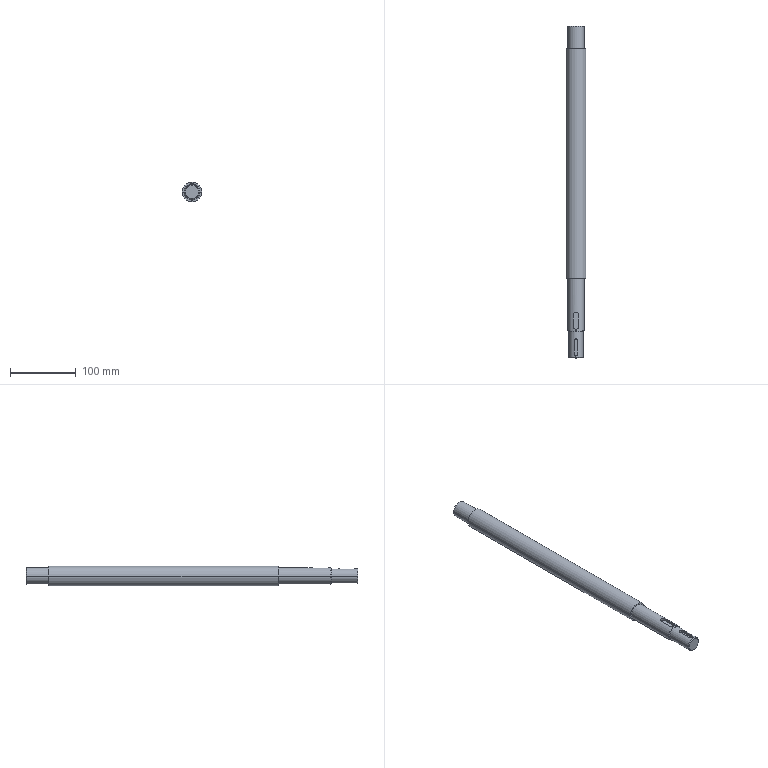Part | STEP file | ROLLER.SHAFT.1.stp | 1 solid | 31 faces | box 30 x 504.3 x 30 mm | volume 316912 mm3 | cylinder 13 | plane 9 | cone 6 | spline 3 | commonest cylinder face diameters 6 x4 25 x4 22 x2 30 x2 8 x1